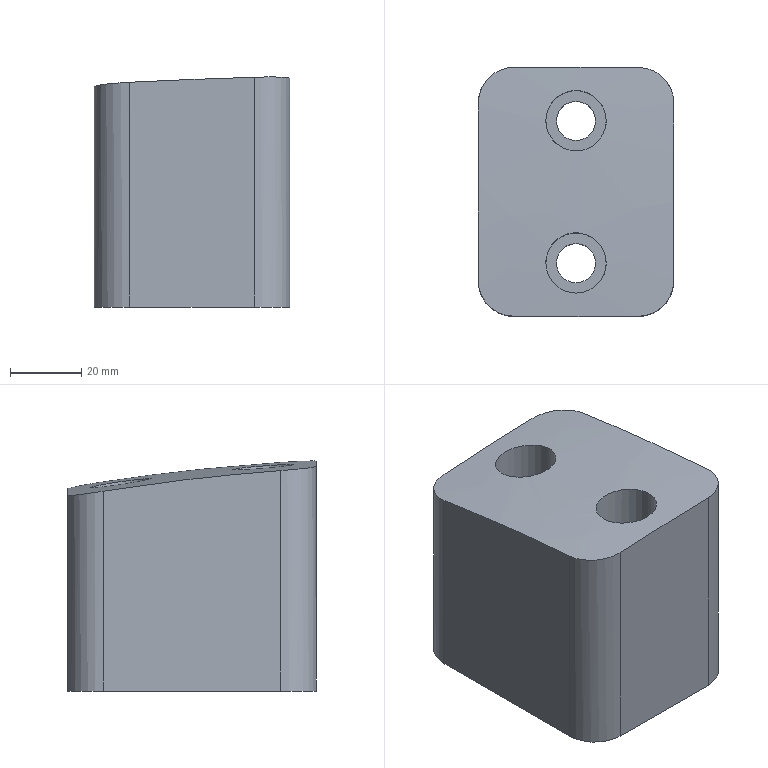Part | NX | features solid 2 | 1 solid | 16 faces | box 55 x 70 x 64.706 mm | volume 206090 mm3 | cylinder 8 | plane 7 | spline 1 | commonest cylinder face diameters 20 x4 11 x2 17 x2
STEP:
#1=CARTESIAN_POINT('',(-88.,285.,-20.));
#2=VERTEX_POINT('',#1);
#3=CARTESIAN_POINT('',(-82.5,285.,-20.));
#4=DIRECTION('',(0.,0.,-1.));
#5=DIRECTION('',(-1.,0.,0.));
#6=AXIS2_PLACEMENT_3D('',#3,#4,#5);
#7=CIRCLE('',#6,5.5);
#8=EDGE_CURVE('',#2,#2,#7,.F.);
#9=ORIENTED_EDGE('',*,*,#8,.T.);
#10=EDGE_LOOP('',(#9));
#11=FACE_BOUND('',#10,.T.);
#12=CARTESIAN_POINT('',(-110.,280.,-20.));
#13=VERTEX_POINT('',#12);
#14=CARTESIAN_POINT('',(-110.,330.,-20.));
#15=VERTEX_POINT('',#14);
#16=CARTESIAN_POINT('',(-110.,290.,-20.));
#17=DIRECTION('',(0.,1.,0.));
#18=VECTOR('',#17,1000.);
#19=LINE('',#16,#18);
#20=EDGE_CURVE('',#13,#15,#19,.T.);
#21=ORIENTED_EDGE('',*,*,#20,.T.);
#22=CARTESIAN_POINT('',(-100.,340.,-20.));
#23=VERTEX_POINT('',#22);
#24=CARTESIAN_POINT('',(-100.,330.,-20.));
#25=DIRECTION('',(0.,0.,-1.));
#26=DIRECTION('',(-1.,0.,0.));
#27=AXIS2_PLACEMENT_3D('',#24,#25,#26);
#28=CIRCLE('',#27,10.);
#29=EDGE_CURVE('',#23,#15,#28,.F.);
#30=ORIENTED_EDGE('',*,*,#29,.F.);
#31=CARTESIAN_POINT('',(-65.,340.,-20.));
#32=VERTEX_POINT('',#31);
#33=CARTESIAN_POINT('',(-55.,340.,-20.));
#34=DIRECTION('',(1.,0.,0.));
#35=VECTOR('',#34,1000.);
#36=LINE('',#33,#35);
#37=EDGE_CURVE('',#32,#23,#36,.F.);
#38=ORIENTED_EDGE('',*,*,#37,.F.);
#39=CARTESIAN_POINT('',(-55.,330.,-20.));
#40=VERTEX_POINT('',#39);
#41=CARTESIAN_POINT('',(-65.,330.,-20.));
#42=DIRECTION('',(0.,0.,-1.));
#43=DIRECTION('',(-1.,0.,0.));
#44=AXIS2_PLACEMENT_3D('',#41,#42,#43);
#45=CIRCLE('',#44,10.);
#46=EDGE_CURVE('',#40,#32,#45,.F.);
#47=ORIENTED_EDGE('',*,*,#46,.F.);
#48=CARTESIAN_POINT('',(-55.,280.,-20.));
#49=VERTEX_POINT('',#48);
#50=CARTESIAN_POINT('',(-55.,290.,-20.));
#51=DIRECTION('',(0.,-1.,0.));
#52=VECTOR('',#51,1000.);
#53=LINE('',#50,#52);
#54=EDGE_CURVE('',#49,#40,#53,.F.);
#55=ORIENTED_EDGE('',*,*,#54,.F.);
#56=CARTESIAN_POINT('',(-65.,270.,-20.));
#57=VERTEX_POINT('',#56);
#58=CARTESIAN_POINT('',(-65.,280.,-20.));
#59=DIRECTION('',(0.,0.,-1.));
#60=DIRECTION('',(-1.,0.,0.));
#61=AXIS2_PLACEMENT_3D('',#58,#59,#60);
#62=CIRCLE('',#61,10.);
#63=EDGE_CURVE('',#57,#49,#62,.F.);
#64=ORIENTED_EDGE('',*,*,#63,.F.);
#65=CARTESIAN_POINT('',(-100.,270.,-20.));
#66=VERTEX_POINT('',#65);
#67=CARTESIAN_POINT('',(-55.,270.,-20.));
#68=DIRECTION('',(-1.,0.,0.));
#69=VECTOR('',#68,1000.);
#70=LINE('',#67,#69);
#71=EDGE_CURVE('',#57,#66,#70,.T.);
#72=ORIENTED_EDGE('',*,*,#71,.T.);
#73=CARTESIAN_POINT('',(-100.,280.,-20.));
#74=DIRECTION('',(0.,0.,-1.));
#75=DIRECTION('',(-1.,0.,0.));
#76=AXIS2_PLACEMENT_3D('',#73,#74,#75);
#77=CIRCLE('',#76,10.);
#78=EDGE_CURVE('',#13,#66,#77,.F.);
#79=ORIENTED_EDGE('',*,*,#78,.F.);
#80=EDGE_LOOP('',(#21,#30,#38,#47,#55,#64,#72,#79));
#81=FACE_BOUND('',#80,.T.);
#82=CARTESIAN_POINT('',(-88.,325.,-20.));
#83=VERTEX_POINT('',#82);
#84=CARTESIAN_POINT('',(-82.5,325.,-20.));
#85=DIRECTION('',(0.,0.,-1.));
#86=DIRECTION('',(-1.,0.,0.));
#87=AXIS2_PLACEMENT_3D('',#84,#85,#86);
#88=CIRCLE('',#87,5.5);
#89=EDGE_CURVE('',#83,#83,#88,.F.);
#90=ORIENTED_EDGE('',*,*,#89,.T.);
#91=EDGE_LOOP('',(#90));
#92=FACE_BOUND('',#91,.T.);
#93=CARTESIAN_POINT('',(-55.,290.,-20.));
#94=DIRECTION('',(0.,0.,1.));
#95=DIRECTION('',(-1.,0.,0.));
#96=AXIS2_PLACEMENT_3D('',#93,#94,#95);
#97=PLANE('',#96);
#98=ADVANCED_FACE('',(#11,#81,#92),#97,.F.);
#99=CARTESIAN_POINT('',(-74.,285.,43.305));
#100=VERTEX_POINT('',#99);
#101=CARTESIAN_POINT('',(-75.842,278.327,43.735));
#102=CARTESIAN_POINT('',(-73.081,285.007,43.351));
#103=CARTESIAN_POINT('',(-75.834,291.646,42.688));
#104=CARTESIAN_POINT('',(-82.469,294.421,42.155));
#105=CARTESIAN_POINT('',(-89.158,291.671,42.111));
#106=CARTESIAN_POINT('',(-91.916,285.001,42.557));
#107=CARTESIAN_POINT('',(-89.178,278.364,43.183));
#108=CARTESIAN_POINT('',(-82.533,275.577,43.654));
#109=CARTESIAN_POINT('',(-75.842,278.327,43.735));
#110=CARTESIAN_POINT('',(-73.081,285.007,43.351));
#111=CARTESIAN_POINT('',(-75.834,291.646,42.688));
#112=B_SPLINE_CURVE_WITH_KNOTS('',3,(#101,#102,#103,#104,#105,#106,#107,#108,#109,#110,#111),.UNSPECIFIED.,.T.,.F.,(1,1,1,1,1,1,1,1,1,1,1,1,1,1,1),(-0.01997,-0.01331,-0.006656,0.,0.006656,0.01331,0.01997,0.02662,0.03328,0.03994,0.04659,0.05325,0.05991,0.06656,0.07322),.UNSPECIFIED.);
#113=EDGE_CURVE('',#100,#100,#112,.T.);
#114=ORIENTED_EDGE('',*,*,#113,.F.);
#115=EDGE_LOOP('',(#114));
#116=FACE_BOUND('',#115,.T.);
#117=CARTESIAN_POINT('',(-100.,270.,43.213));
#118=VERTEX_POINT('',#117);
#119=CARTESIAN_POINT('',(-65.,270.,44.631));
#120=VERTEX_POINT('',#119);
#121=CARTESIAN_POINT('',(-100.,270.,43.213));
#122=CARTESIAN_POINT('',(-88.338,270.,43.792));
#123=CARTESIAN_POINT('',(-76.671,270.,44.263));
#124=CARTESIAN_POINT('',(-65.,270.,44.631));
#125=B_SPLINE_CURVE_WITH_KNOTS('',3,(#121,#122,#123,#124),.UNSPECIFIED.,.F.,.F.,(4,4),(0.01001,0.04504),.UNSPECIFIED.);
#126=EDGE_CURVE('',#118,#120,#125,.T.);
#127=ORIENTED_EDGE('',*,*,#126,.T.);
#128=CARTESIAN_POINT('',(-55.,280.,44.291));
#129=VERTEX_POINT('',#128);
#130=CARTESIAN_POINT('',(-55.,280.,44.291));
#131=CARTESIAN_POINT('',(-55.,277.364,44.475));
#132=CARTESIAN_POINT('',(-57.167,272.187,44.745));
#133=CARTESIAN_POINT('',(-62.358,270.,44.714));
#134=CARTESIAN_POINT('',(-65.,270.,44.631));
#135=B_SPLINE_CURVE_WITH_KNOTS('',3,(#130,#131,#132,#133,#134),.UNSPECIFIED.,.F.,.F.,(4,1,4),(0.,0.007816,0.01563),.UNSPECIFIED.);
#136=EDGE_CURVE('',#129,#120,#135,.T.);
#137=ORIENTED_EDGE('',*,*,#136,.F.);
#138=CARTESIAN_POINT('',(-55.,330.,38.832));
#139=VERTEX_POINT('',#138);
#140=CARTESIAN_POINT('',(-55.,280.,44.291));
#141=CARTESIAN_POINT('',(-55.,296.716,43.125));
#142=CARTESIAN_POINT('',(-55.,313.421,41.376));
#143=CARTESIAN_POINT('',(-55.,330.,38.832));
#144=B_SPLINE_CURVE_WITH_KNOTS('',3,(#140,#141,#142,#143),.UNSPECIFIED.,.F.,.F.,(4,4),(-0.01003,0.04027),.UNSPECIFIED.);
#145=EDGE_CURVE('',#129,#139,#144,.T.);
#146=ORIENTED_EDGE('',*,*,#145,.T.);
#147=CARTESIAN_POINT('',(-65.,340.,36.842));
#148=VERTEX_POINT('',#147);
#149=CARTESIAN_POINT('',(-65.,340.,36.842));
#150=CARTESIAN_POINT('',(-62.338,340.,36.945));
#151=CARTESIAN_POINT('',(-57.155,337.791,37.52));
#152=CARTESIAN_POINT('',(-55.,332.633,38.428));
#153=CARTESIAN_POINT('',(-55.,330.,38.832));
#154=B_SPLINE_CURVE_WITH_KNOTS('',3,(#149,#150,#151,#152,#153),.UNSPECIFIED.,.F.,.F.,(4,1,4),(0.,0.007878,0.01576),.UNSPECIFIED.);
#155=EDGE_CURVE('',#148,#139,#154,.T.);
#156=ORIENTED_EDGE('',*,*,#155,.F.);
#157=CARTESIAN_POINT('',(-100.,340.,35.12));
#158=VERTEX_POINT('',#157);
#159=CARTESIAN_POINT('',(-65.,340.,36.842));
#160=CARTESIAN_POINT('',(-76.673,340.,36.395));
#161=CARTESIAN_POINT('',(-88.34,340.,35.823));
#162=CARTESIAN_POINT('',(-100.,340.,35.12));
#163=B_SPLINE_CURVE_WITH_KNOTS('',3,(#159,#160,#161,#162),.UNSPECIFIED.,.F.,.F.,(4,4),(0.01001,0.04505),.UNSPECIFIED.);
#164=EDGE_CURVE('',#148,#158,#163,.T.);
#165=ORIENTED_EDGE('',*,*,#164,.T.);
#166=CARTESIAN_POINT('',(-110.,330.,36.195));
#167=VERTEX_POINT('',#166);
#168=CARTESIAN_POINT('',(-110.,330.,36.195));
#169=CARTESIAN_POINT('',(-110.,332.619,35.774));
#170=CARTESIAN_POINT('',(-107.864,337.786,35.035));
#171=CARTESIAN_POINT('',(-102.649,340.,34.961));
#172=CARTESIAN_POINT('',(-100.,340.,35.12));
#173=B_SPLINE_CURVE_WITH_KNOTS('',3,(#168,#169,#170,#171,#172),.UNSPECIFIED.,.F.,.F.,(4,1,4),(0.,0.007847,0.01569),.UNSPECIFIED.);
#174=EDGE_CURVE('',#167,#158,#173,.T.);
#175=ORIENTED_EDGE('',*,*,#174,.F.);
#176=CARTESIAN_POINT('',(-110.,280.,41.998));
#177=VERTEX_POINT('',#176);
#178=CARTESIAN_POINT('',(-110.,330.,36.195));
#179=CARTESIAN_POINT('',(-110.,313.427,38.858));
#180=CARTESIAN_POINT('',(-110.,296.721,40.723));
#181=CARTESIAN_POINT('',(-110.,280.,41.998));
#182=B_SPLINE_CURVE_WITH_KNOTS('',3,(#178,#179,#180,#181),.UNSPECIFIED.,.F.,.F.,(4,4),(0.01014,0.06048),.UNSPECIFIED.);
#183=EDGE_CURVE('',#167,#177,#182,.T.);
#184=ORIENTED_EDGE('',*,*,#183,.T.);
#185=CARTESIAN_POINT('',(-100.,270.,43.213));
#186=CARTESIAN_POINT('',(-102.646,270.,43.082));
#187=CARTESIAN_POINT('',(-107.82,272.179,42.683));
#188=CARTESIAN_POINT('',(-110.,277.359,42.199));
#189=CARTESIAN_POINT('',(-110.,280.,41.998));
#190=B_SPLINE_CURVE_WITH_KNOTS('',3,(#185,#186,#187,#188,#189),.UNSPECIFIED.,.F.,.F.,(4,1,4),(0.,0.007834,0.01567),.UNSPECIFIED.);
#191=EDGE_CURVE('',#118,#177,#190,.T.);
#192=ORIENTED_EDGE('',*,*,#191,.F.);
#193=EDGE_LOOP('',(#127,#137,#146,#156,#165,#175,#184,#192));
#194=FACE_BOUND('',#193,.T.);
#195=CARTESIAN_POINT('',(-74.,325.,38.881));
#196=VERTEX_POINT('',#195);
#197=CARTESIAN_POINT('',(-75.827,318.334,39.742));
#198=CARTESIAN_POINT('',(-73.09,325.013,38.934));
#199=CARTESIAN_POINT('',(-75.812,331.615,37.808));
#200=CARTESIAN_POINT('',(-82.442,334.43,37.037));
#201=CARTESIAN_POINT('',(-89.171,331.665,37.156));
#202=CARTESIAN_POINT('',(-91.907,325.004,38.047));
#203=CARTESIAN_POINT('',(-89.202,318.395,39.117));
#204=CARTESIAN_POINT('',(-82.56,315.568,39.803));
#205=CARTESIAN_POINT('',(-75.827,318.334,39.742));
#206=CARTESIAN_POINT('',(-73.09,325.013,38.934));
#207=CARTESIAN_POINT('',(-75.812,331.615,37.808));
#208=B_SPLINE_CURVE_WITH_KNOTS('',3,(#197,#198,#199,#200,#201,#202,#203,#204,#205,#206,#207),.UNSPECIFIED.,.T.,.F.,(1,1,1,1,1,1,1,1,1,1,1,1,1,1,1),(-0.02004,-0.01336,-0.006681,0.,0.006681,0.01336,0.02004,0.02673,0.03341,0.04009,0.04677,0.05345,0.06013,0.06681,0.07349),.UNSPECIFIED.);
#209=EDGE_CURVE('',#196,#196,#208,.T.);
#210=ORIENTED_EDGE('',*,*,#209,.F.);
#211=EDGE_LOOP('',(#210));
#212=FACE_BOUND('',#211,.T.);
#213=CARTESIAN_POINT('',(-52.783,342.899,36.753));
#214=CARTESIAN_POINT('',(-64.245,342.48,36.471));
#215=CARTESIAN_POINT('',(-75.683,341.954,36.11));
#216=CARTESIAN_POINT('',(-87.095,341.325,35.668));
#217=CARTESIAN_POINT('',(-98.479,340.591,35.146));
#218=CARTESIAN_POINT('',(-109.833,339.749,34.542));
#219=CARTESIAN_POINT('',(-53.186,329.497,39.152));
#220=CARTESIAN_POINT('',(-64.731,329.072,38.867));
#221=CARTESIAN_POINT('',(-76.25,328.541,38.501));
#222=CARTESIAN_POINT('',(-87.738,327.906,38.055));
#223=CARTESIAN_POINT('',(-99.195,327.166,37.527));
#224=CARTESIAN_POINT('',(-110.62,326.319,36.917));
#225=CARTESIAN_POINT('',(-53.599,315.542,41.167));
#226=CARTESIAN_POINT('',(-65.23,315.113,40.879));
#227=CARTESIAN_POINT('',(-76.831,314.577,40.51));
#228=CARTESIAN_POINT('',(-88.399,313.936,40.061));
#229=CARTESIAN_POINT('',(-99.931,313.191,39.529));
#230=CARTESIAN_POINT('',(-111.427,312.338,38.916));
#231=CARTESIAN_POINT('',(-54.023,300.994,42.797));
#232=CARTESIAN_POINT('',(-65.742,300.561,42.507));
#233=CARTESIAN_POINT('',(-77.428,300.019,42.137));
#234=CARTESIAN_POINT('',(-89.076,299.374,41.685));
#235=CARTESIAN_POINT('',(-100.685,298.624,41.152));
#236=CARTESIAN_POINT('',(-112.254,297.765,40.537));
#237=CARTESIAN_POINT('',(-54.457,285.8,44.048));
#238=CARTESIAN_POINT('',(-66.266,285.363,43.757));
#239=CARTESIAN_POINT('',(-78.039,284.817,43.386));
#240=CARTESIAN_POINT('',(-89.771,284.167,42.935));
#241=CARTESIAN_POINT('',(-101.459,283.412,42.401));
#242=CARTESIAN_POINT('',(-113.103,282.549,41.787));
#243=CARTESIAN_POINT('',(-54.901,269.903,44.929));
#244=CARTESIAN_POINT('',(-66.802,269.463,44.639));
#245=CARTESIAN_POINT('',(-78.664,268.913,44.268));
#246=CARTESIAN_POINT('',(-90.481,268.259,43.817));
#247=CARTESIAN_POINT('',(-102.251,267.5,43.286));
#248=CARTESIAN_POINT('',(-113.973,266.632,42.674));
#249=B_SPLINE_SURFACE_WITH_KNOTS('',5,5,((#213,#214,#215,#216,#217,#218),(#219,#220,#221,#222,#223,#224),(#225,#226,#227,#228,#229,#230),(#231,#232,#233,#234,#235,#236),(#237,#238,#239,#240,#241,#242),(#243,#244,#245,#246,#247,#248)),.UNSPECIFIED.,.F.,.F.,.F.,(6,6),(6,6),(0.2914,0.4126),(0.2198,0.4593),.PIECEWISE_BEZIER_KNOTS.);
#250=ADVANCED_FACE('',(#116,#194,#212),#249,.F.);
#251=ORIENTED_EDGE('',*,*,#54,.T.);
#252=CARTESIAN_POINT('',(-55.,330.,-10.));
#253=DIRECTION('',(0.,0.,-1.));
#254=VECTOR('',#253,1000.);
#255=LINE('',#252,#254);
#256=EDGE_CURVE('',#139,#40,#255,.T.);
#257=ORIENTED_EDGE('',*,*,#256,.F.);
#258=ORIENTED_EDGE('',*,*,#145,.F.);
#259=CARTESIAN_POINT('',(-55.,280.,-10.));
#260=DIRECTION('',(0.,0.,1.));
#261=VECTOR('',#260,1000.);
#262=LINE('',#259,#261);
#263=EDGE_CURVE('',#49,#129,#262,.T.);
#264=ORIENTED_EDGE('',*,*,#263,.F.);
#265=EDGE_LOOP('',(#251,#257,#258,#264));
#266=FACE_BOUND('',#265,.T.);
#267=CARTESIAN_POINT('',(-55.,290.,-10.));
#268=DIRECTION('',(-1.,0.,0.));
#269=DIRECTION('',(0.,1.,0.));
#270=AXIS2_PLACEMENT_3D('',#267,#268,#269);
#271=PLANE('',#270);
#272=ADVANCED_FACE('',(#266),#271,.F.);
#273=ORIENTED_EDGE('',*,*,#164,.F.);
#274=CARTESIAN_POINT('',(-65.,340.,-10.));
#275=DIRECTION('',(0.,0.,-1.));
#276=VECTOR('',#275,1000.);
#277=LINE('',#274,#276);
#278=EDGE_CURVE('',#32,#148,#277,.F.);
#279=ORIENTED_EDGE('',*,*,#278,.F.);
#280=ORIENTED_EDGE('',*,*,#37,.T.);
#281=CARTESIAN_POINT('',(-100.,340.,-10.));
#282=DIRECTION('',(0.,0.,1.));
#283=VECTOR('',#282,1000.);
#284=LINE('',#281,#283);
#285=EDGE_CURVE('',#158,#23,#284,.F.);
#286=ORIENTED_EDGE('',*,*,#285,.F.);
#287=EDGE_LOOP('',(#273,#279,#280,#286));
#288=FACE_BOUND('',#287,.T.);
#289=CARTESIAN_POINT('',(-55.,340.,-10.));
#290=DIRECTION('',(0.,-1.,0.));
#291=DIRECTION('',(-1.,0.,0.));
#292=AXIS2_PLACEMENT_3D('',#289,#290,#291);
#293=PLANE('',#292);
#294=ADVANCED_FACE('',(#288),#293,.F.);
#295=ORIENTED_EDGE('',*,*,#183,.F.);
#296=CARTESIAN_POINT('',(-110.,330.,-10.));
#297=DIRECTION('',(0.,0.,-1.));
#298=VECTOR('',#297,1000.);
#299=LINE('',#296,#298);
#300=EDGE_CURVE('',#15,#167,#299,.F.);
#301=ORIENTED_EDGE('',*,*,#300,.F.);
#302=ORIENTED_EDGE('',*,*,#20,.F.);
#303=CARTESIAN_POINT('',(-110.,280.,-10.));
#304=DIRECTION('',(0.,0.,1.));
#305=VECTOR('',#304,1000.);
#306=LINE('',#303,#305);
#307=EDGE_CURVE('',#177,#13,#306,.F.);
#308=ORIENTED_EDGE('',*,*,#307,.F.);
#309=EDGE_LOOP('',(#295,#301,#302,#308));
#310=FACE_BOUND('',#309,.T.);
#311=CARTESIAN_POINT('',(-110.,290.,-10.));
#312=DIRECTION('',(-1.,0.,0.));
#313=DIRECTION('',(0.,1.,0.));
#314=AXIS2_PLACEMENT_3D('',#311,#312,#313);
#315=PLANE('',#314);
#316=ADVANCED_FACE('',(#310),#315,.T.);
#317=ORIENTED_EDGE('',*,*,#71,.F.);
#318=CARTESIAN_POINT('',(-65.,270.,-10.));
#319=DIRECTION('',(0.,0.,-1.));
#320=VECTOR('',#319,1000.);
#321=LINE('',#318,#320);
#322=EDGE_CURVE('',#120,#57,#321,.T.);
#323=ORIENTED_EDGE('',*,*,#322,.F.);
#324=ORIENTED_EDGE('',*,*,#126,.F.);
#325=CARTESIAN_POINT('',(-100.,270.,-10.));
#326=DIRECTION('',(0.,0.,1.));
#327=VECTOR('',#326,1000.);
#328=LINE('',#325,#327);
#329=EDGE_CURVE('',#66,#118,#328,.T.);
#330=ORIENTED_EDGE('',*,*,#329,.F.);
#331=EDGE_LOOP('',(#317,#323,#324,#330));
#332=FACE_BOUND('',#331,.T.);
#333=CARTESIAN_POINT('',(-55.,270.,-10.));
#334=DIRECTION('',(0.,-1.,0.));
#335=DIRECTION('',(-1.,0.,0.));
#336=AXIS2_PLACEMENT_3D('',#333,#334,#335);
#337=PLANE('',#336);
#338=ADVANCED_FACE('',(#332),#337,.T.);
#339=CARTESIAN_POINT('',(-88.,285.,0.));
#340=VERTEX_POINT('',#339);
#341=CARTESIAN_POINT('',(-82.5,285.,0.));
#342=DIRECTION('',(0.,0.,-1.));
#343=DIRECTION('',(-1.,0.,0.));
#344=AXIS2_PLACEMENT_3D('',#341,#342,#343);
#345=CIRCLE('',#344,5.5);
#346=EDGE_CURVE('',#340,#340,#345,.F.);
#347=ORIENTED_EDGE('',*,*,#346,.T.);
#348=EDGE_LOOP('',(#347));
#349=FACE_BOUND('',#348,.T.);
#350=ORIENTED_EDGE('',*,*,#8,.F.);
#351=EDGE_LOOP('',(#350));
#352=FACE_BOUND('',#351,.T.);
#353=CARTESIAN_POINT('',(-82.5,285.,80.));
#354=DIRECTION('',(0.,0.,-1.));
#355=DIRECTION('',(1.,0.,0.));
#356=AXIS2_PLACEMENT_3D('',#353,#354,#355);
#357=CYLINDRICAL_SURFACE('',#356,5.5);
#358=ADVANCED_FACE('',(#349,#352),#357,.F.);
#359=CARTESIAN_POINT('',(-91.,285.,0.));
#360=VERTEX_POINT('',#359);
#361=CARTESIAN_POINT('',(-82.5,285.,0.));
#362=DIRECTION('',(0.,0.,-1.));
#363=DIRECTION('',(-1.,0.,0.));
#364=AXIS2_PLACEMENT_3D('',#361,#362,#363);
#365=CIRCLE('',#364,8.5);
#366=EDGE_CURVE('',#360,#360,#365,.T.);
#367=ORIENTED_EDGE('',*,*,#366,.F.);
#368=EDGE_LOOP('',(#367));
#369=FACE_BOUND('',#368,.T.);
#370=ORIENTED_EDGE('',*,*,#346,.F.);
#371=EDGE_LOOP('',(#370));
#372=FACE_BOUND('',#371,.T.);
#373=CARTESIAN_POINT('',(-82.5,285.,0.));
#374=DIRECTION('',(0.,0.,1.));
#375=DIRECTION('',(-1.,0.,0.));
#376=AXIS2_PLACEMENT_3D('',#373,#374,#375);
#377=PLANE('',#376);
#378=ADVANCED_FACE('',(#369,#372),#377,.T.);
#379=ORIENTED_EDGE('',*,*,#113,.T.);
#380=EDGE_LOOP('',(#379));
#381=FACE_BOUND('',#380,.T.);
#382=ORIENTED_EDGE('',*,*,#366,.T.);
#383=EDGE_LOOP('',(#382));
#384=FACE_BOUND('',#383,.T.);
#385=CARTESIAN_POINT('',(-82.5,285.,180.));
#386=DIRECTION('',(0.,0.,-1.));
#387=DIRECTION('',(1.,0.,0.));
#388=AXIS2_PLACEMENT_3D('',#385,#386,#387);
#389=CYLINDRICAL_SURFACE('',#388,8.5);
#390=ADVANCED_FACE('',(#381,#384),#389,.F.);
#391=CARTESIAN_POINT('',(-88.,325.,0.));
#392=VERTEX_POINT('',#391);
#393=CARTESIAN_POINT('',(-82.5,325.,0.));
#394=DIRECTION('',(0.,0.,-1.));
#395=DIRECTION('',(-1.,0.,0.));
#396=AXIS2_PLACEMENT_3D('',#393,#394,#395);
#397=CIRCLE('',#396,5.5);
#398=EDGE_CURVE('',#392,#392,#397,.F.);
#399=ORIENTED_EDGE('',*,*,#398,.T.);
#400=EDGE_LOOP('',(#399));
#401=FACE_BOUND('',#400,.T.);
#402=ORIENTED_EDGE('',*,*,#89,.F.);
#403=EDGE_LOOP('',(#402));
#404=FACE_BOUND('',#403,.T.);
#405=CARTESIAN_POINT('',(-82.5,325.,80.));
#406=DIRECTION('',(0.,0.,-1.));
#407=DIRECTION('',(1.,0.,0.));
#408=AXIS2_PLACEMENT_3D('',#405,#406,#407);
#409=CYLINDRICAL_SURFACE('',#408,5.5);
#410=ADVANCED_FACE('',(#401,#404),#409,.F.);
#411=CARTESIAN_POINT('',(-91.,325.,0.));
#412=VERTEX_POINT('',#411);
#413=CARTESIAN_POINT('',(-82.5,325.,0.));
#414=DIRECTION('',(0.,0.,-1.));
#415=DIRECTION('',(-1.,0.,0.));
#416=AXIS2_PLACEMENT_3D('',#413,#414,#415);
#417=CIRCLE('',#416,8.5);
#418=EDGE_CURVE('',#412,#412,#417,.T.);
#419=ORIENTED_EDGE('',*,*,#418,.F.);
#420=EDGE_LOOP('',(#419));
#421=FACE_BOUND('',#420,.T.);
#422=ORIENTED_EDGE('',*,*,#398,.F.);
#423=EDGE_LOOP('',(#422));
#424=FACE_BOUND('',#423,.T.);
#425=CARTESIAN_POINT('',(-82.5,325.,0.));
#426=DIRECTION('',(0.,0.,1.));
#427=DIRECTION('',(-1.,0.,0.));
#428=AXIS2_PLACEMENT_3D('',#425,#426,#427);
#429=PLANE('',#428);
#430=ADVANCED_FACE('',(#421,#424),#429,.T.);
#431=ORIENTED_EDGE('',*,*,#209,.T.);
#432=EDGE_LOOP('',(#431));
#433=FACE_BOUND('',#432,.T.);
#434=ORIENTED_EDGE('',*,*,#418,.T.);
#435=EDGE_LOOP('',(#434));
#436=FACE_BOUND('',#435,.T.);
#437=CARTESIAN_POINT('',(-82.5,325.,180.));
#438=DIRECTION('',(0.,0.,-1.));
#439=DIRECTION('',(1.,0.,0.));
#440=AXIS2_PLACEMENT_3D('',#437,#438,#439);
#441=CYLINDRICAL_SURFACE('',#440,8.5);
#442=ADVANCED_FACE('',(#433,#436),#441,.F.);
#443=ORIENTED_EDGE('',*,*,#78,.T.);
#444=ORIENTED_EDGE('',*,*,#329,.T.);
#445=ORIENTED_EDGE('',*,*,#191,.T.);
#446=ORIENTED_EDGE('',*,*,#307,.T.);
#447=EDGE_LOOP('',(#443,#444,#445,#446));
#448=FACE_BOUND('',#447,.T.);
#449=CARTESIAN_POINT('',(-100.,280.,-10.));
#450=DIRECTION('',(0.,0.,1.));
#451=DIRECTION('',(-1.,0.,0.));
#452=AXIS2_PLACEMENT_3D('',#449,#450,#451);
#453=CYLINDRICAL_SURFACE('',#452,10.);
#454=ADVANCED_FACE('',(#448),#453,.T.);
#455=ORIENTED_EDGE('',*,*,#63,.T.);
#456=ORIENTED_EDGE('',*,*,#263,.T.);
#457=ORIENTED_EDGE('',*,*,#136,.T.);
#458=ORIENTED_EDGE('',*,*,#322,.T.);
#459=EDGE_LOOP('',(#455,#456,#457,#458));
#460=FACE_BOUND('',#459,.T.);
#461=CARTESIAN_POINT('',(-65.,280.,-10.));
#462=DIRECTION('',(0.,0.,-1.));
#463=DIRECTION('',(1.,0.,0.));
#464=AXIS2_PLACEMENT_3D('',#461,#462,#463);
#465=CYLINDRICAL_SURFACE('',#464,10.);
#466=ADVANCED_FACE('',(#460),#465,.T.);
#467=ORIENTED_EDGE('',*,*,#29,.T.);
#468=ORIENTED_EDGE('',*,*,#300,.T.);
#469=ORIENTED_EDGE('',*,*,#174,.T.);
#470=ORIENTED_EDGE('',*,*,#285,.T.);
#471=EDGE_LOOP('',(#467,#468,#469,#470));
#472=FACE_BOUND('',#471,.T.);
#473=CARTESIAN_POINT('',(-100.,330.,-10.));
#474=DIRECTION('',(0.,0.,-1.));
#475=DIRECTION('',(1.,0.,0.));
#476=AXIS2_PLACEMENT_3D('',#473,#474,#475);
#477=CYLINDRICAL_SURFACE('',#476,10.);
#478=ADVANCED_FACE('',(#472),#477,.T.);
#479=ORIENTED_EDGE('',*,*,#46,.T.);
#480=ORIENTED_EDGE('',*,*,#278,.T.);
#481=ORIENTED_EDGE('',*,*,#155,.T.);
#482=ORIENTED_EDGE('',*,*,#256,.T.);
#483=EDGE_LOOP('',(#479,#480,#481,#482));
#484=FACE_BOUND('',#483,.T.);
#485=CARTESIAN_POINT('',(-65.,330.,-10.));
#486=DIRECTION('',(0.,0.,1.));
#487=DIRECTION('',(-1.,0.,0.));
#488=AXIS2_PLACEMENT_3D('',#485,#486,#487);
#489=CYLINDRICAL_SURFACE('',#488,10.);
#490=ADVANCED_FACE('',(#484),#489,.T.);
#491=CLOSED_SHELL('',(#98,#250,#272,#294,#316,#338,#358,#378,#390,#410,#430,#442,#454,#466,#478,#490));
#492=MANIFOLD_SOLID_BREP('',#491);
#493=(LENGTH_UNIT()NAMED_UNIT(*)SI_UNIT(.MILLI.,.METRE.));
#494=UNCERTAINTY_MEASURE_WITH_UNIT(LENGTH_MEASURE(0.0508),#493,'','');
#495=(NAMED_UNIT(*)PLANE_ANGLE_UNIT()SI_UNIT($,.RADIAN.));
#496=(NAMED_UNIT(*)SI_UNIT($,.STERADIAN.)SOLID_ANGLE_UNIT());
#497=(GEOMETRIC_REPRESENTATION_CONTEXT(3)GLOBAL_UNCERTAINTY_ASSIGNED_CONTEXT((#494))GLOBAL_UNIT_ASSIGNED_CONTEXT((#493,#495,#496))REPRESENTATION_CONTEXT('',''));
#498=ADVANCED_BREP_SHAPE_REPRESENTATION('',(#492),#497);